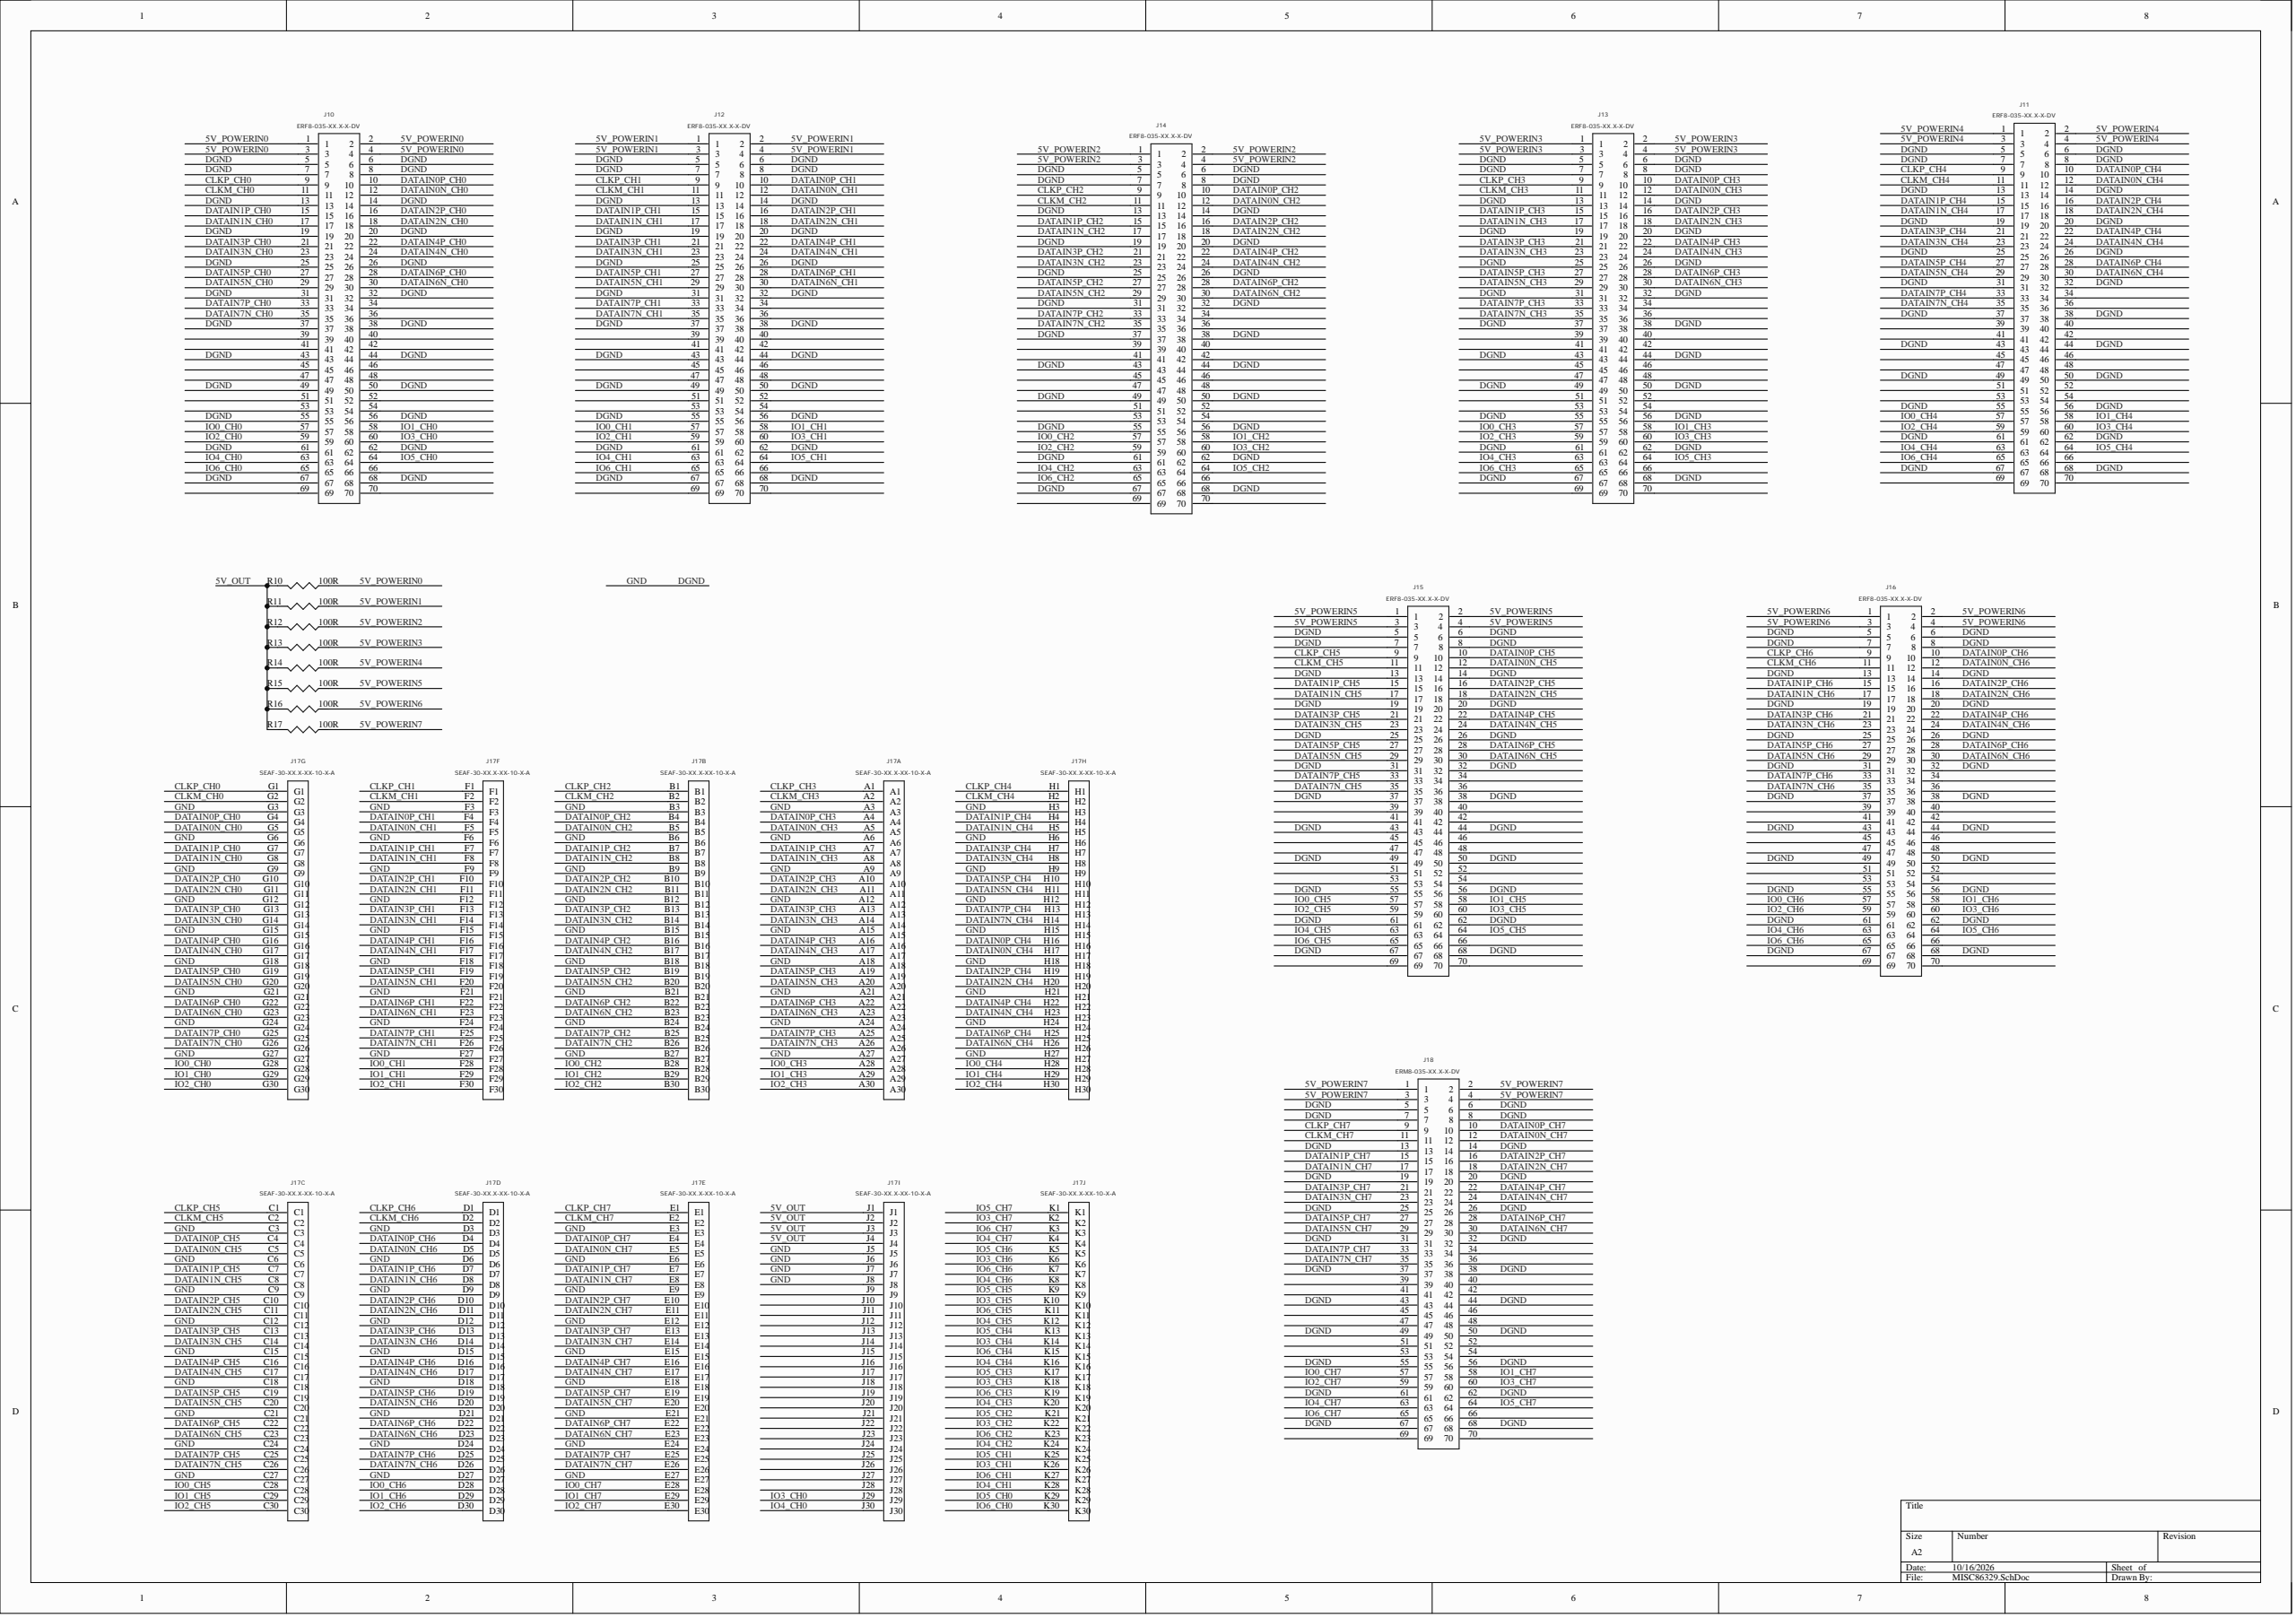Circuit board | Altium Designer | 17 parts | 210 nets
Bill of materials:
Comment,Description,Designator,Footprint,LibRef,Quantity
"ERF8-035-XX.X-X-DV","0.8mm Edge Rate Socket Assembly, Double Vertical Row, 30 Positions Per Row.","J10, J11, J12, J13, J14, J15, J16","ERF8-035-XX.X-X-DV","ERF8-035-XX.X-X-DV","7"
"SEAF-30-XX.X-XX-10-X-A","Socket Array Assembly, Surface Mount, 0.050"" Pitch, 300 Pins","J17","SEAF-30-XX.X-XX-10-X-A","SEAF-30-XX.X-XX-10-X-A","1"
"ERM8-035-XX.X-X-DV","0.8mm Edge Rate Terminal Assembly, Double Vertical Row, 40 Position, 0.8mm Pitch","J18","ERF8-035-XX.X-X-DV","ERM8-035-XX.X-X-DV","1"
"100R","Resistor","R10, R11, R12, R13, R14, R15, R16, R17","R1210","Res_4K7_0.05_1608[0603]_FENGHUA","8"
Netlist (Protel format):
[
J10
ERF8-035-XX.X-X-DV
ERF8-035-XX.X-X-DV



]
[
J11
ERF8-035-XX.X-X-DV
ERF8-035-XX.X-X-DV



]
[
J12
ERF8-035-XX.X-X-DV
ERF8-035-XX.X-X-DV



]
[
J13
ERF8-035-XX.X-X-DV
ERF8-035-XX.X-X-DV



]
[
J14
ERF8-035-XX.X-X-DV
ERF8-035-XX.X-X-DV



]
[
J15
ERF8-035-XX.X-X-DV
ERF8-035-XX.X-X-DV



]
[
J16
ERF8-035-XX.X-X-DV
ERF8-035-XX.X-X-DV



]
[
J17
SEAF-30-XX.X-XX-10-X-A
SEAF-30-XX.X-XX-10-X-A



]
[
J18
ERF8-035-XX.X-X-DV
ERM8-035-XX.X-X-DV



]
[
R10
R1210
100R



]
[
R11
R1210
100R



]
[
R12
R1210
100R



]
[
R13
R1210
100R



]
[
R14
R1210
100R



]
[
R15
R1210
100R



]
[
R16
R1210
100R



]
[
R17
R1210
100R



]
(
IO6_CH7
J17-K3
J18-65
)
(
IO6_CH6
J16-65
J17-K7
)
(
IO6_CH5
J15-65
J17-K11
)
(
IO6_CH4
J11-65
J17-K15
)
(
IO6_CH3
J13-65
J17-K19
)
(
IO6_CH2
J14-65
J17-K23
)
(
IO6_CH1
J12-65
J17-K27
)
(
IO6_CH0
J10-65
J17-K30
)
(
IO5_CH7
J17-K1
J18-64
)
(
IO5_CH6
J16-64
J17-K5
)
(
IO5_CH5
J15-64
J17-K9
)
(
IO5_CH4
J11-64
J17-K13
)
(
IO5_CH3
J13-64
J17-K17
)
(
IO5_CH2
J14-64
J17-K21
)
(
IO5_CH1
J12-64
J17-K25
)
(
IO5_CH0
J10-64
J17-K29
)
(
IO4_CH7
J17-K4
J18-63
)
(
IO4_CH6
J16-63
J17-K8
)
(
IO4_CH5
J15-63
J17-K12
)
(
IO4_CH4
J11-63
J17-K16
)
(
IO4_CH3
J13-63
J17-K20
)
(
IO4_CH2
J14-63
J17-K24
)
(
IO4_CH1
J12-63
J17-K28
)
(
IO4_CH0
J10-63
J17-J30
)
(
IO3_CH7
J17-K2
J18-60
)
(
IO3_CH6
J16-60
J17-K6
)
(
IO3_CH5
J15-60
J17-K10
)
(
IO3_CH4
J11-60
J17-K14
)
(
IO3_CH3
J13-60
J17-K18
)
(
IO3_CH2
J14-60
J17-K22
)
(
IO3_CH1
J12-60
J17-K26
)
(
IO3_CH0
J10-60
J17-J29
)
(
IO2_CH7
J17-E30
J18-59
)
(
IO2_CH6
J16-59
J17-D30
)
(
IO2_CH5
J15-59
J17-C30
)
(
IO2_CH4
J11-59
J17-H30
)
(
IO2_CH3
J13-59
J17-A30
)
(
IO2_CH2
J14-59
J17-B30
)
(
IO2_CH1
J12-59
J17-F30
)
(
IO2_CH0
J10-59
J17-G30
)
(
IO1_CH7
J17-E29
J18-58
)
(
IO1_CH6
J16-58
J17-D29
)
(
IO1_CH5
J15-58
J17-C29
)
(
IO1_CH4
J11-58
J17-H29
)
(
IO1_CH3
J13-58
J17-A29
)
(
IO1_CH2
J14-58
J17-B29
)
(
IO1_CH1
J12-58
J17-F29
)
(
IO1_CH0
J10-58
J17-G29
)
(
IO0_CH7
J17-E28
J18-57
)
(
IO0_CH6
J16-57
J17-D28
)
(
IO0_CH5
J15-57
J17-C28
)
(
IO0_CH4
J11-57
J17-H28
)
(
IO0_CH3
J13-57
J17-A28
)
(
IO0_CH2
J14-57
J17-B28
)
(
IO0_CH1
J12-57
J17-F28
)
(
IO0_CH0
J10-57
J17-G28
)
(
DGND
J10-5
J10-6
J10-7
J10-8
J10-13
J10-14
J10-19
J10-20
J10-25
J10-26
J10-31
J10-32
J10-37
J10-38
J10-43
J10-44
J10-49
J10-50
J10-55
J10-56
J10-61
J10-62
J10-67
J10-68
J11-5
J11-6
J11-7
J11-8
J11-13
J11-14
J11-19
J11-20
J11-25
J11-26
J11-31
J11-32
J11-37
J11-38
J11-43
J11-44
J11-49
J11-50
J11-55
J11-56
J11-61
J11-62
J11-67
J11-68
J12-5
J12-6
J12-7
J12-8
J12-13
J12-14
J12-19
J12-20
J12-25
J12-26
J12-31
J12-32
J12-37
J12-38
J12-43
J12-44
J12-49
J12-50
J12-55
J12-56
J12-61
J12-62
J12-67
J12-68
J13-5
J13-6
J13-7
J13-8
J13-13
J13-14
J13-19
J13-20
J13-25
J13-26
J13-31
J13-32
J13-37
J13-38
J13-43
J13-44
J13-49
J13-50
J13-55
J13-56
J13-61
J13-62
J13-67
J13-68
J14-5
J14-6
J14-7
J14-8
J14-13
J14-14
J14-19
J14-20
J14-25
J14-26
J14-31
J14-32
J14-37
J14-38
J14-43
J14-44
J14-49
J14-50
J14-55
J14-56
J14-61
J14-62
J14-67
J14-68
J15-5
J15-6
J15-7
J15-8
J15-13
J15-14
J15-19
J15-20
J15-25
J15-26
J15-31
J15-32
J15-37
J15-38
J15-43
J15-44
J15-49
J15-50
J15-55
J15-56
J15-61
J15-62
J15-67
J15-68
J16-5
J16-6
J16-7
J16-8
J16-13
J16-14
J16-19
J16-20
J16-25
J16-26
J16-31
J16-32
J16-37
J16-38
J16-43
J16-44
J16-49
J16-50
J16-55
J16-56
J16-61
J16-62
J16-67
J16-68
J17-A3
J17-A6
J17-A9
J17-A12
J17-A15
J17-A18
J17-A21
J17-A24
J17-A27
J17-B3
J17-B6
J17-B9
J17-B12
J17-B15
J17-B18
J17-B21
J17-B24
J17-B27
J17-C3
J17-C6
J17-C9
J17-C12
J17-C15
J17-C18
J17-C21
J17-C24
J17-C27
J17-D3
J17-D6
J17-D9
J17-D12
J17-D15
J17-D18
J17-D21
J17-D24
J17-D27
J17-E3
J17-E6
J17-E9
J17-E12
J17-E15
J17-E18
J17-E21
J17-E24
J17-E27
J17-F3
J17-F6
J17-F9
J17-F12
J17-F15
J17-F18
J17-F21
J17-F24
J17-F27
J17-G3
J17-G6
J17-G9
J17-G12
J17-G15
J17-G18
J17-G21
J17-G24
J17-G27
J17-H3
J17-H6
J17-H9
J17-H12
J17-H15
J17-H18
J17-H21
J17-H24
J17-H27
J17-J5
J17-J6
J17-J7
J17-J8
J18-5
J18-6
J18-7
J18-8
J18-13
J18-14
J18-19
J18-20
J18-25
J18-26
J18-31
J18-32
J18-37
J18-38
J18-43
J18-44
J18-49
J18-50
J18-55
J18-56
J18-61
J18-62
J18-67
J18-68
)
(
DATAIN7P_CH7
J17-E25
J18-33
)
(
DATAIN7P_CH6
J16-33
J17-D25
)
(
DATAIN7P_CH5
J15-33
J17-C25
)
(
DATAIN7P_CH4
J11-33
J17-H13
)
(
DATAIN7P_CH3
J13-33
J17-A25
)
(
DATAIN7P_CH2
J14-33
J17-B25
)
(
DATAIN7P_CH1
J12-33
J17-F25
)
(
DATAIN7P_CH0
J10-33
J17-G25
)
(
DATAIN7N_CH7
J17-E26
J18-35
)
(
DATAIN7N_CH6
J16-35
J17-D26
)
(
DATAIN7N_CH5
J15-35
J17-C26
)
(
DATAIN7N_CH4
J11-35
J17-H14
)
(
DATAIN7N_CH3
J13-35
J17-A26
)
(
DATAIN7N_CH2
J14-35
J17-B26
)
(
DATAIN7N_CH1
J12-35
J17-F26
)
(
DATAIN7N_CH0
J10-35
J17-G26
)
(
DATAIN6P_CH7
J17-E22
J18-28
)
(
DATAIN6P_CH6
J16-28
J17-D22
)
(
DATAIN6P_CH5
J15-28
J17-C22
)
(
DATAIN6P_CH4
J11-28
J17-H25
)
(
DATAIN6P_CH3
J13-28
J17-A22
)
(
DATAIN6P_CH2
J14-28
J17-B22
)
(
DATAIN6P_CH1
J12-28
J17-F22
)
(
DATAIN6P_CH0
J10-28
J17-G22
)
(
DATAIN6N_CH7
J17-E23
J18-30
)
(
DATAIN6N_CH6
J16-30
J17-D23
)
(
DATAIN6N_CH5
J15-30
J17-C23
)
(
DATAIN6N_CH4
J11-30
J17-H26
)
(
DATAIN6N_CH3
J13-30
J17-A23
)
(
DATAIN6N_CH2
J14-30
J17-B23
)
(
DATAIN6N_CH1
J12-30
J17-F23
)
(
DATAIN6N_CH0
J10-30
J17-G23
)
(
DATAIN5P_CH7
J17-E19
J18-27
)
(
DATAIN5P_CH6
J16-27
J17-D19
)
(
DATAIN5P_CH5
J15-27
J17-C19
)
(
DATAIN5P_CH4
J11-27
J17-H10
)
(
DATAIN5P_CH3
J13-27
J17-A19
)
(
DATAIN5P_CH2
J14-27
J17-B19
)
(
DATAIN5P_CH1
J12-27
J17-F19
)
(
DATAIN5P_CH0
J10-27
J17-G19
)
(
DATAIN5N_CH7
J17-E20
J18-29
)
(
DATAIN5N_CH6
J16-29
J17-D20
)
(
DATAIN5N_CH5
J15-29
J17-C20
)
(
DATAIN5N_CH4
J11-29
J17-H11
)
(
DATAIN5N_CH3
J13-29
J17-A20
)
(
DATAIN5N_CH2
J14-29
J17-B20
)
(
DATAIN5N_CH1
J12-29
J17-F20
)
(
DATAIN5N_CH0
J10-29
J17-G20
)
(
DATAIN4P_CH7
J17-E16
J18-22
)
(
DATAIN4P_CH6
J16-22
J17-D16
)
(
DATAIN4P_CH5
J15-22
J17-C16
)
(
DATAIN4P_CH4
J11-22
J17-H22
)
(
DATAIN4P_CH3
J13-22
J17-A16
)
(
DATAIN4P_CH2
J14-22
J17-B16
)
(
DATAIN4P_CH1
J12-22
J17-F16
)
(
DATAIN4P_CH0
J10-22
J17-G16
)
(
DATAIN4N_CH7
J17-E17
J18-24
)
(
DATAIN4N_CH6
J16-24
J17-D17
)
(
DATAIN4N_CH5
J15-24
J17-C17
)
(
DATAIN4N_CH4
J11-24
J17-H23
)
(
DATAIN4N_CH3
J13-24
J17-A17
)
(
DATAIN4N_CH2
J14-24
J17-B17
)
(
DATAIN4N_CH1
J12-24
J17-F17
)
(
DATAIN4N_CH0
J10-24
J17-G17
)
(
DATAIN3P_CH7
J17-E13
J18-21
)
(
DATAIN3P_CH6
J16-21
J17-D13
)
(
DATAIN3P_CH5
J15-21
J17-C13
)
(
DATAIN3P_CH4
J11-21
J17-H7
)
(
DATAIN3P_CH3
J13-21
J17-A13
)
(
DATAIN3P_CH2
J14-21
J17-B13
)
(
DATAIN3P_CH1
J12-21
J17-F13
)
(
DATAIN3P_CH0
J10-21
J17-G13
)
(
DATAIN3N_CH7
J17-E14
J18-23
)
(
DATAIN3N_CH6
J16-23
J17-D14
)
(
DATAIN3N_CH5
J15-23
J17-C14
)
(
DATAIN3N_CH4
J11-23
J17-H8
)
(
DATAIN3N_CH3
J13-23
J17-A14
)
(
DATAIN3N_CH2
J14-23
J17-B14
)
(
DATAIN3N_CH1
J12-23
J17-F14
)
(
DATAIN3N_CH0
J10-23
J17-G14
)
(
DATAIN2P_CH7
J17-E10
J18-16
)
(
DATAIN2P_CH6
J16-16
J17-D10
)
(
DATAIN2P_CH5
J15-16
J17-C10
)
(
DATAIN2P_CH4
J11-16
J17-H19
)
(
DATAIN2P_CH3
J13-16
J17-A10
)
(
DATAIN2P_CH2
J14-16
J17-B10
)
(
DATAIN2P_CH1
J12-16
J17-F10
)
(
DATAIN2P_CH0
J10-16
J17-G10
)
(
DATAIN2N_CH7
J17-E11
J18-18
)
(
DATAIN2N_CH6
J16-18
J17-D11
)
(
DATAIN2N_CH5
J15-18
J17-C11
)
(
DATAIN2N_CH4
J11-18
J17-H20
)
(
DATAIN2N_CH3
J13-18
J17-A11
)
(
DATAIN2N_CH2
J14-18
J17-B11
)
(
DATAIN2N_CH1
J12-18
J17-F11
)
(
DATAIN2N_CH0
J10-18
J17-G11
)
(
DATAIN1P_CH7
J17-E7
J18-15
)
(
DATAIN1P_CH6
J16-15
J17-D7
)
(
DATAIN1P_CH5
J15-15
J17-C7
)
(
DATAIN1P_CH4
J11-15
J17-H4
)
(
DATAIN1P_CH3
J13-15
J17-A7
)
(
DATAIN1P_CH2
J14-15
J17-B7
)
(
DATAIN1P_CH1
J12-15
J17-F7
)
(
DATAIN1P_CH0
J10-15
J17-G7
)
(
DATAIN1N_CH7
J17-E8
J18-17
)
(
DATAIN1N_CH6
J16-17
J17-D8
)
(
DATAIN1N_CH5
J15-17
J17-C8
)
(
DATAIN1N_CH4
J11-17
J17-H5
)
(
DATAIN1N_CH3
J13-17
J17-A8
)
(
DATAIN1N_CH2
J14-17
J17-B8
)
(
DATAIN1N_CH1
J12-17
J17-F8
)
(
DATAIN1N_CH0
J10-17
J17-G8
)
(
DATAIN0P_CH7
J17-E4
J18-10
)
(
DATAIN0P_CH6
J16-10
J17-D4
)
(
DATAIN0P_CH5
J15-10
J17-C4
)
(
DATAIN0P_CH4
J11-10
J17-H16
)
(
DATAIN0P_CH3
J13-10
J17-A4
)
(
DATAIN0P_CH2
J14-10
J17-B4
)
(
DATAIN0P_CH1
J12-10
J17-F4
)
(
DATAIN0P_CH0
J10-10
J17-G4
)
(
DATAIN0N_CH7
J17-E5
J18-12
)
(
DATAIN0N_CH6
J16-12
J17-D5
)
(
DATAIN0N_CH5
J15-12
J17-C5
)
(
DATAIN0N_CH4
J11-12
J17-H17
)
(
DATAIN0N_CH3
J13-12
J17-A5
)
(
DATAIN0N_CH2
J14-12
J17-B5
)
(
DATAIN0N_CH1
J12-12
J17-F5
)
(
DATAIN0N_CH0
J10-12
J17-G5
)
(
CLKP_CH7
J17-E1
J18-9
)
(
CLKP_CH6
J16-9
J17-D1
)
(
CLKP_CH5
J15-9
J17-C1
)
(
CLKP_CH4
J11-9
J17-H1
)
(
CLKP_CH3
J13-9
J17-A1
)
(
CLKP_CH2
J14-9
J17-B1
)
(
CLKP_CH1
J12-9
J17-F1
)
(
CLKP_CH0
J10-9
J17-G1
)
(
CLKM_CH7
J17-E2
J18-11
)
(
CLKM_CH6
J16-11
J17-D2
)
(
CLKM_CH5
J15-11
J17-C2
)
(
CLKM_CH4
J11-11
J17-H2
)
(
CLKM_CH3
J13-11
J17-A2
)
(
CLKM_CH2
J14-11
J17-B2
)
(
CLKM_CH1
J12-11
J17-F2
)
(
CLKM_CH0
J10-11
J17-G2
)
(
5V_POWERIN7
J18-1
J18-2
J18-3
J18-4
R17-1
)
(
5V_POWERIN6
J16-1
J16-2
J16-3
J16-4
R16-1
)
(
5V_POWERIN5
J15-1
J15-2
J15-3
J15-4
R15-1
)
(
5V_POWERIN4
J11-1
J11-2
J11-3
J11-4
R14-1
)
(
5V_POWERIN3
J13-1
J13-2
J13-3
J13-4
R13-1
)
(
5V_POWERIN2
J14-1
J14-2
J14-3
J14-4
R12-1
)
(
5V_POWERIN1
J12-1
J12-2
J12-3
J12-4
R11-1
)
(
5V_POWERIN0
J10-1
J10-2
J10-3
J10-4
R10-1
)
(
5V_OUT
J17-J1
J17-J2
J17-J3
J17-J4
R10-2
R11-2
R12-2
R13-2
R14-2
R15-2
R16-2
R17-2
)